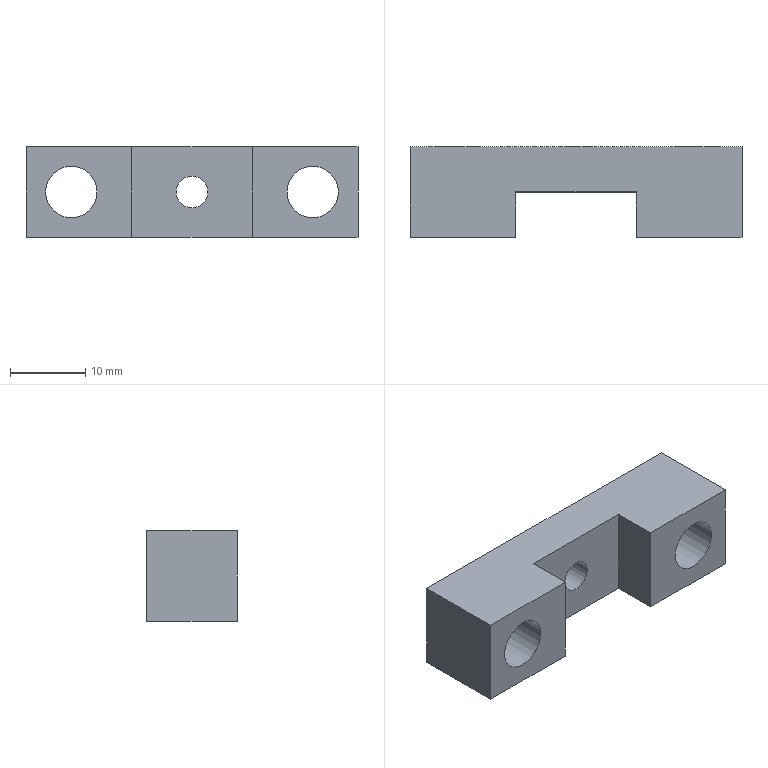Part | NX | features BREP 1 | 1 solid | 13 faces | box 44 x 12 x 12 mm | volume 4229 mm3 | plane 10 | cylinder 3 | commonest cylinder face diameters 6.8 x2 4.2 x1
STEP:
#1=CARTESIAN_POINT('',(16.,-6.,9.4));
#2=VERTEX_POINT('',#1);
#3=CARTESIAN_POINT('',(16.,-6.,6.));
#4=DIRECTION('',(0.,1.,0.));
#5=DIRECTION('',(0.,0.,1.));
#6=AXIS2_PLACEMENT_3D('',#3,#4,#5);
#7=CIRCLE('',#6,3.4);
#8=EDGE_CURVE('',#2,#2,#7,.T.);
#9=ORIENTED_EDGE('',*,*,#8,.T.);
#10=EDGE_LOOP('',(#9));
#11=FACE_BOUND('',#10,.T.);
#12=CARTESIAN_POINT('',(8.,-6.,12.));
#13=VERTEX_POINT('',#12);
#14=CARTESIAN_POINT('',(22.,-6.,12.));
#15=VERTEX_POINT('',#14);
#16=CARTESIAN_POINT('',(-22.,-6.,12.));
#17=DIRECTION('',(1.,0.,0.));
#18=VECTOR('',#17,1000.);
#19=LINE('',#16,#18);
#20=EDGE_CURVE('',#13,#15,#19,.T.);
#21=ORIENTED_EDGE('',*,*,#20,.F.);
#22=CARTESIAN_POINT('',(8.,-6.,0.));
#23=VERTEX_POINT('',#22);
#24=CARTESIAN_POINT('',(8.,-6.,0.));
#25=DIRECTION('',(0.,0.,1.));
#26=VECTOR('',#25,1000.);
#27=LINE('',#24,#26);
#28=EDGE_CURVE('',#23,#13,#27,.T.);
#29=ORIENTED_EDGE('',*,*,#28,.F.);
#30=CARTESIAN_POINT('',(22.,-6.,0.));
#31=VERTEX_POINT('',#30);
#32=CARTESIAN_POINT('',(-22.,-6.,0.));
#33=DIRECTION('',(1.,0.,0.));
#34=VECTOR('',#33,1000.);
#35=LINE('',#32,#34);
#36=EDGE_CURVE('',#23,#31,#35,.T.);
#37=ORIENTED_EDGE('',*,*,#36,.T.);
#38=CARTESIAN_POINT('',(22.,-6.,12.));
#39=DIRECTION('',(0.,0.,-1.));
#40=VECTOR('',#39,1000.);
#41=LINE('',#38,#40);
#42=EDGE_CURVE('',#15,#31,#41,.T.);
#43=ORIENTED_EDGE('',*,*,#42,.F.);
#44=EDGE_LOOP('',(#21,#29,#37,#43));
#45=FACE_BOUND('',#44,.T.);
#46=CARTESIAN_POINT('',(-22.,-6.,12.));
#47=DIRECTION('',(0.,1.,0.));
#48=DIRECTION('',(0.,0.,-1.));
#49=AXIS2_PLACEMENT_3D('',#46,#47,#48);
#50=PLANE('',#49);
#51=ADVANCED_FACE('',(#11,#45),#50,.F.);
#52=CARTESIAN_POINT('',(22.,6.,0.));
#53=VERTEX_POINT('',#52);
#54=CARTESIAN_POINT('',(22.,6.,0.));
#55=DIRECTION('',(0.,1.,0.));
#56=VECTOR('',#55,1000.);
#57=LINE('',#54,#56);
#58=EDGE_CURVE('',#31,#53,#57,.T.);
#59=ORIENTED_EDGE('',*,*,#58,.T.);
#60=CARTESIAN_POINT('',(22.,6.,12.));
#61=VERTEX_POINT('',#60);
#62=CARTESIAN_POINT('',(22.,6.,12.));
#63=DIRECTION('',(0.,0.,-1.));
#64=VECTOR('',#63,1000.);
#65=LINE('',#62,#64);
#66=EDGE_CURVE('',#61,#53,#65,.T.);
#67=ORIENTED_EDGE('',*,*,#66,.F.);
#68=CARTESIAN_POINT('',(22.,6.,12.));
#69=DIRECTION('',(0.,1.,0.));
#70=VECTOR('',#69,1000.);
#71=LINE('',#68,#70);
#72=EDGE_CURVE('',#15,#61,#71,.T.);
#73=ORIENTED_EDGE('',*,*,#72,.F.);
#74=ORIENTED_EDGE('',*,*,#42,.T.);
#75=EDGE_LOOP('',(#59,#67,#73,#74));
#76=FACE_BOUND('',#75,.T.);
#77=CARTESIAN_POINT('',(22.,6.,12.));
#78=DIRECTION('',(-1.,0.,0.));
#79=DIRECTION('',(0.,0.,-1.));
#80=AXIS2_PLACEMENT_3D('',#77,#78,#79);
#81=PLANE('',#80);
#82=ADVANCED_FACE('',(#76),#81,.F.);
#83=CARTESIAN_POINT('',(0.,6.,3.9));
#84=VERTEX_POINT('',#83);
#85=CARTESIAN_POINT('',(0.,6.,6.));
#86=DIRECTION('',(0.,-1.,0.));
#87=DIRECTION('',(0.,0.,-1.));
#88=AXIS2_PLACEMENT_3D('',#85,#86,#87);
#89=CIRCLE('',#88,2.1);
#90=EDGE_CURVE('',#84,#84,#89,.T.);
#91=ORIENTED_EDGE('',*,*,#90,.T.);
#92=EDGE_LOOP('',(#91));
#93=FACE_BOUND('',#92,.T.);
#94=CARTESIAN_POINT('',(16.,6.,9.4));
#95=VERTEX_POINT('',#94);
#96=CARTESIAN_POINT('',(16.,6.,6.));
#97=DIRECTION('',(0.,1.,0.));
#98=DIRECTION('',(0.,0.,1.));
#99=AXIS2_PLACEMENT_3D('',#96,#97,#98);
#100=CIRCLE('',#99,3.4);
#101=EDGE_CURVE('',#95,#95,#100,.T.);
#102=ORIENTED_EDGE('',*,*,#101,.F.);
#103=EDGE_LOOP('',(#102));
#104=FACE_BOUND('',#103,.T.);
#105=CARTESIAN_POINT('',(-16.,6.,9.4));
#106=VERTEX_POINT('',#105);
#107=CARTESIAN_POINT('',(-16.,6.,6.));
#108=DIRECTION('',(0.,1.,0.));
#109=DIRECTION('',(0.,0.,1.));
#110=AXIS2_PLACEMENT_3D('',#107,#108,#109);
#111=CIRCLE('',#110,3.4);
#112=EDGE_CURVE('',#106,#106,#111,.T.);
#113=ORIENTED_EDGE('',*,*,#112,.F.);
#114=EDGE_LOOP('',(#113));
#115=FACE_BOUND('',#114,.T.);
#116=CARTESIAN_POINT('',(-22.,6.,0.));
#117=VERTEX_POINT('',#116);
#118=CARTESIAN_POINT('',(-22.,6.,0.));
#119=DIRECTION('',(-1.,0.,0.));
#120=VECTOR('',#119,1000.);
#121=LINE('',#118,#120);
#122=EDGE_CURVE('',#53,#117,#121,.T.);
#123=ORIENTED_EDGE('',*,*,#122,.T.);
#124=CARTESIAN_POINT('',(-22.,6.,12.));
#125=VERTEX_POINT('',#124);
#126=CARTESIAN_POINT('',(-22.,6.,12.));
#127=DIRECTION('',(0.,0.,-1.));
#128=VECTOR('',#127,1000.);
#129=LINE('',#126,#128);
#130=EDGE_CURVE('',#125,#117,#129,.T.);
#131=ORIENTED_EDGE('',*,*,#130,.F.);
#132=CARTESIAN_POINT('',(-22.,6.,12.));
#133=DIRECTION('',(-1.,0.,0.));
#134=VECTOR('',#133,1000.);
#135=LINE('',#132,#134);
#136=EDGE_CURVE('',#61,#125,#135,.T.);
#137=ORIENTED_EDGE('',*,*,#136,.F.);
#138=ORIENTED_EDGE('',*,*,#66,.T.);
#139=EDGE_LOOP('',(#123,#131,#137,#138));
#140=FACE_BOUND('',#139,.T.);
#141=CARTESIAN_POINT('',(-22.,6.,12.));
#142=DIRECTION('',(0.,-1.,0.));
#143=DIRECTION('',(0.,0.,1.));
#144=AXIS2_PLACEMENT_3D('',#141,#142,#143);
#145=PLANE('',#144);
#146=ADVANCED_FACE('',(#93,#104,#115,#140),#145,.F.);
#147=CARTESIAN_POINT('',(-22.,-6.,0.));
#148=VERTEX_POINT('',#147);
#149=CARTESIAN_POINT('',(-22.,6.,0.));
#150=DIRECTION('',(0.,-1.,0.));
#151=VECTOR('',#150,1000.);
#152=LINE('',#149,#151);
#153=EDGE_CURVE('',#117,#148,#152,.T.);
#154=ORIENTED_EDGE('',*,*,#153,.T.);
#155=CARTESIAN_POINT('',(-22.,-6.,12.));
#156=VERTEX_POINT('',#155);
#157=CARTESIAN_POINT('',(-22.,-6.,12.));
#158=DIRECTION('',(0.,0.,-1.));
#159=VECTOR('',#158,1000.);
#160=LINE('',#157,#159);
#161=EDGE_CURVE('',#156,#148,#160,.T.);
#162=ORIENTED_EDGE('',*,*,#161,.F.);
#163=CARTESIAN_POINT('',(-22.,6.,12.));
#164=DIRECTION('',(0.,-1.,0.));
#165=VECTOR('',#164,1000.);
#166=LINE('',#163,#165);
#167=EDGE_CURVE('',#125,#156,#166,.T.);
#168=ORIENTED_EDGE('',*,*,#167,.F.);
#169=ORIENTED_EDGE('',*,*,#130,.T.);
#170=EDGE_LOOP('',(#154,#162,#168,#169));
#171=FACE_BOUND('',#170,.T.);
#172=CARTESIAN_POINT('',(-22.,6.,12.));
#173=DIRECTION('',(1.,0.,0.));
#174=DIRECTION('',(0.,0.,1.));
#175=AXIS2_PLACEMENT_3D('',#172,#173,#174);
#176=PLANE('',#175);
#177=ADVANCED_FACE('',(#171),#176,.F.);
#178=CARTESIAN_POINT('',(-16.,-6.,9.4));
#179=VERTEX_POINT('',#178);
#180=CARTESIAN_POINT('',(-16.,-6.,6.));
#181=DIRECTION('',(0.,1.,0.));
#182=DIRECTION('',(0.,0.,1.));
#183=AXIS2_PLACEMENT_3D('',#180,#181,#182);
#184=CIRCLE('',#183,3.4);
#185=EDGE_CURVE('',#179,#179,#184,.T.);
#186=ORIENTED_EDGE('',*,*,#185,.T.);
#187=EDGE_LOOP('',(#186));
#188=FACE_BOUND('',#187,.T.);
#189=CARTESIAN_POINT('',(-8.,-6.,0.));
#190=VERTEX_POINT('',#189);
#191=CARTESIAN_POINT('',(-22.,-6.,0.));
#192=DIRECTION('',(1.,0.,0.));
#193=VECTOR('',#192,1000.);
#194=LINE('',#191,#193);
#195=EDGE_CURVE('',#148,#190,#194,.T.);
#196=ORIENTED_EDGE('',*,*,#195,.T.);
#197=CARTESIAN_POINT('',(-8.,-6.,12.));
#198=VERTEX_POINT('',#197);
#199=CARTESIAN_POINT('',(-8.,-6.,0.));
#200=DIRECTION('',(0.,0.,-1.));
#201=VECTOR('',#200,1000.);
#202=LINE('',#199,#201);
#203=EDGE_CURVE('',#198,#190,#202,.T.);
#204=ORIENTED_EDGE('',*,*,#203,.F.);
#205=CARTESIAN_POINT('',(-22.,-6.,12.));
#206=DIRECTION('',(1.,0.,0.));
#207=VECTOR('',#206,1000.);
#208=LINE('',#205,#207);
#209=EDGE_CURVE('',#156,#198,#208,.T.);
#210=ORIENTED_EDGE('',*,*,#209,.F.);
#211=ORIENTED_EDGE('',*,*,#161,.T.);
#212=EDGE_LOOP('',(#196,#204,#210,#211));
#213=FACE_BOUND('',#212,.T.);
#214=CARTESIAN_POINT('',(-22.,-6.,12.));
#215=DIRECTION('',(0.,1.,0.));
#216=DIRECTION('',(0.,0.,-1.));
#217=AXIS2_PLACEMENT_3D('',#214,#215,#216);
#218=PLANE('',#217);
#219=ADVANCED_FACE('',(#188,#213),#218,.F.);
#220=CARTESIAN_POINT('',(8.,0.,12.));
#221=VERTEX_POINT('',#220);
#222=CARTESIAN_POINT('',(8.,0.,12.));
#223=DIRECTION('',(0.,-1.,0.));
#224=VECTOR('',#223,1000.);
#225=LINE('',#222,#224);
#226=EDGE_CURVE('',#221,#13,#225,.T.);
#227=ORIENTED_EDGE('',*,*,#226,.T.);
#228=ORIENTED_EDGE('',*,*,#20,.T.);
#229=ORIENTED_EDGE('',*,*,#72,.T.);
#230=ORIENTED_EDGE('',*,*,#136,.T.);
#231=ORIENTED_EDGE('',*,*,#167,.T.);
#232=ORIENTED_EDGE('',*,*,#209,.T.);
#233=CARTESIAN_POINT('',(-8.,0.,12.));
#234=VERTEX_POINT('',#233);
#235=CARTESIAN_POINT('',(-8.,0.,12.));
#236=DIRECTION('',(0.,-1.,0.));
#237=VECTOR('',#236,1000.);
#238=LINE('',#235,#237);
#239=EDGE_CURVE('',#234,#198,#238,.T.);
#240=ORIENTED_EDGE('',*,*,#239,.F.);
#241=CARTESIAN_POINT('',(-8.,0.,12.));
#242=DIRECTION('',(-1.,0.,0.));
#243=VECTOR('',#242,1000.);
#244=LINE('',#241,#243);
#245=EDGE_CURVE('',#221,#234,#244,.T.);
#246=ORIENTED_EDGE('',*,*,#245,.F.);
#247=EDGE_LOOP('',(#227,#228,#229,#230,#231,#232,#240,#246));
#248=FACE_BOUND('',#247,.T.);
#249=CARTESIAN_POINT('',(0.,0.,12.));
#250=DIRECTION('',(0.,0.,1.));
#251=DIRECTION('',(-1.,0.,0.));
#252=AXIS2_PLACEMENT_3D('',#249,#250,#251);
#253=PLANE('',#252);
#254=ADVANCED_FACE('',(#248),#253,.T.);
#255=ORIENTED_EDGE('',*,*,#36,.F.);
#256=CARTESIAN_POINT('',(8.,0.,0.));
#257=VERTEX_POINT('',#256);
#258=CARTESIAN_POINT('',(8.,0.,0.));
#259=DIRECTION('',(0.,-1.,0.));
#260=VECTOR('',#259,1000.);
#261=LINE('',#258,#260);
#262=EDGE_CURVE('',#257,#23,#261,.T.);
#263=ORIENTED_EDGE('',*,*,#262,.F.);
#264=CARTESIAN_POINT('',(-8.,0.,0.));
#265=VERTEX_POINT('',#264);
#266=CARTESIAN_POINT('',(-8.,0.,0.));
#267=DIRECTION('',(1.,0.,0.));
#268=VECTOR('',#267,1000.);
#269=LINE('',#266,#268);
#270=EDGE_CURVE('',#265,#257,#269,.T.);
#271=ORIENTED_EDGE('',*,*,#270,.F.);
#272=CARTESIAN_POINT('',(-8.,0.,0.));
#273=DIRECTION('',(0.,-1.,0.));
#274=VECTOR('',#273,1000.);
#275=LINE('',#272,#274);
#276=EDGE_CURVE('',#265,#190,#275,.T.);
#277=ORIENTED_EDGE('',*,*,#276,.T.);
#278=ORIENTED_EDGE('',*,*,#195,.F.);
#279=ORIENTED_EDGE('',*,*,#153,.F.);
#280=ORIENTED_EDGE('',*,*,#122,.F.);
#281=ORIENTED_EDGE('',*,*,#58,.F.);
#282=EDGE_LOOP('',(#255,#263,#271,#277,#278,#279,#280,#281));
#283=FACE_BOUND('',#282,.T.);
#284=CARTESIAN_POINT('',(0.,0.,0.));
#285=DIRECTION('',(0.,0.,1.));
#286=DIRECTION('',(-1.,0.,0.));
#287=AXIS2_PLACEMENT_3D('',#284,#285,#286);
#288=PLANE('',#287);
#289=ADVANCED_FACE('',(#283),#288,.F.);
#290=ORIENTED_EDGE('',*,*,#28,.T.);
#291=ORIENTED_EDGE('',*,*,#226,.F.);
#292=CARTESIAN_POINT('',(8.,0.,0.));
#293=DIRECTION('',(0.,0.,1.));
#294=VECTOR('',#293,1000.);
#295=LINE('',#292,#294);
#296=EDGE_CURVE('',#257,#221,#295,.T.);
#297=ORIENTED_EDGE('',*,*,#296,.F.);
#298=ORIENTED_EDGE('',*,*,#262,.T.);
#299=EDGE_LOOP('',(#290,#291,#297,#298));
#300=FACE_BOUND('',#299,.T.);
#301=CARTESIAN_POINT('',(8.,0.,0.));
#302=DIRECTION('',(1.,0.,0.));
#303=DIRECTION('',(0.,0.,1.));
#304=AXIS2_PLACEMENT_3D('',#301,#302,#303);
#305=PLANE('',#304);
#306=ADVANCED_FACE('',(#300),#305,.F.);
#307=ORIENTED_EDGE('',*,*,#203,.T.);
#308=ORIENTED_EDGE('',*,*,#276,.F.);
#309=CARTESIAN_POINT('',(-8.,0.,0.));
#310=DIRECTION('',(0.,0.,-1.));
#311=VECTOR('',#310,1000.);
#312=LINE('',#309,#311);
#313=EDGE_CURVE('',#234,#265,#312,.T.);
#314=ORIENTED_EDGE('',*,*,#313,.F.);
#315=ORIENTED_EDGE('',*,*,#239,.T.);
#316=EDGE_LOOP('',(#307,#308,#314,#315));
#317=FACE_BOUND('',#316,.T.);
#318=CARTESIAN_POINT('',(-8.,0.,0.));
#319=DIRECTION('',(-1.,0.,0.));
#320=DIRECTION('',(0.,0.,-1.));
#321=AXIS2_PLACEMENT_3D('',#318,#319,#320);
#322=PLANE('',#321);
#323=ADVANCED_FACE('',(#317),#322,.F.);
#324=CARTESIAN_POINT('',(0.,0.,3.9));
#325=VERTEX_POINT('',#324);
#326=CARTESIAN_POINT('',(0.,0.,6.));
#327=DIRECTION('',(0.,-1.,0.));
#328=DIRECTION('',(0.,0.,-1.));
#329=AXIS2_PLACEMENT_3D('',#326,#327,#328);
#330=CIRCLE('',#329,2.1);
#331=EDGE_CURVE('',#325,#325,#330,.T.);
#332=ORIENTED_EDGE('',*,*,#331,.F.);
#333=EDGE_LOOP('',(#332));
#334=FACE_BOUND('',#333,.T.);
#335=ORIENTED_EDGE('',*,*,#296,.T.);
#336=ORIENTED_EDGE('',*,*,#245,.T.);
#337=ORIENTED_EDGE('',*,*,#313,.T.);
#338=ORIENTED_EDGE('',*,*,#270,.T.);
#339=EDGE_LOOP('',(#335,#336,#337,#338));
#340=FACE_BOUND('',#339,.T.);
#341=CARTESIAN_POINT('',(0.,0.,0.));
#342=DIRECTION('',(0.,1.,0.));
#343=DIRECTION('',(0.,0.,-1.));
#344=AXIS2_PLACEMENT_3D('',#341,#342,#343);
#345=PLANE('',#344);
#346=ADVANCED_FACE('',(#334,#340),#345,.F.);
#347=ORIENTED_EDGE('',*,*,#185,.F.);
#348=EDGE_LOOP('',(#347));
#349=FACE_BOUND('',#348,.T.);
#350=ORIENTED_EDGE('',*,*,#112,.T.);
#351=EDGE_LOOP('',(#350));
#352=FACE_BOUND('',#351,.T.);
#353=CARTESIAN_POINT('',(-16.,6.,6.));
#354=DIRECTION('',(0.,1.,0.));
#355=DIRECTION('',(0.,0.,-1.));
#356=AXIS2_PLACEMENT_3D('',#353,#354,#355);
#357=CYLINDRICAL_SURFACE('',#356,3.4);
#358=ADVANCED_FACE('',(#349,#352),#357,.F.);
#359=ORIENTED_EDGE('',*,*,#8,.F.);
#360=EDGE_LOOP('',(#359));
#361=FACE_BOUND('',#360,.T.);
#362=ORIENTED_EDGE('',*,*,#101,.T.);
#363=EDGE_LOOP('',(#362));
#364=FACE_BOUND('',#363,.T.);
#365=CARTESIAN_POINT('',(16.,6.,6.));
#366=DIRECTION('',(0.,1.,0.));
#367=DIRECTION('',(0.,0.,-1.));
#368=AXIS2_PLACEMENT_3D('',#365,#366,#367);
#369=CYLINDRICAL_SURFACE('',#368,3.4);
#370=ADVANCED_FACE('',(#361,#364),#369,.F.);
#371=ORIENTED_EDGE('',*,*,#90,.F.);
#372=EDGE_LOOP('',(#371));
#373=FACE_BOUND('',#372,.T.);
#374=ORIENTED_EDGE('',*,*,#331,.T.);
#375=EDGE_LOOP('',(#374));
#376=FACE_BOUND('',#375,.T.);
#377=CARTESIAN_POINT('',(0.,0.,6.));
#378=DIRECTION('',(0.,-1.,0.));
#379=DIRECTION('',(0.,0.,1.));
#380=AXIS2_PLACEMENT_3D('',#377,#378,#379);
#381=CYLINDRICAL_SURFACE('',#380,2.1);
#382=ADVANCED_FACE('',(#373,#376),#381,.F.);
#383=CLOSED_SHELL('',(#51,#82,#146,#177,#219,#254,#289,#306,#323,#346,#358,#370,#382));
#384=MANIFOLD_SOLID_BREP('',#383);
#385=(LENGTH_UNIT()NAMED_UNIT(*)SI_UNIT(.MILLI.,.METRE.));
#386=UNCERTAINTY_MEASURE_WITH_UNIT(LENGTH_MEASURE(0.00001),#385,'','');
#387=(NAMED_UNIT(*)PLANE_ANGLE_UNIT()SI_UNIT($,.RADIAN.));
#388=(NAMED_UNIT(*)SI_UNIT($,.STERADIAN.)SOLID_ANGLE_UNIT());
#389=(GEOMETRIC_REPRESENTATION_CONTEXT(3)GLOBAL_UNCERTAINTY_ASSIGNED_CONTEXT((#386))GLOBAL_UNIT_ASSIGNED_CONTEXT((#385,#387,#388))REPRESENTATION_CONTEXT('',''));
#390=ADVANCED_BREP_SHAPE_REPRESENTATION('',(#384),#389);